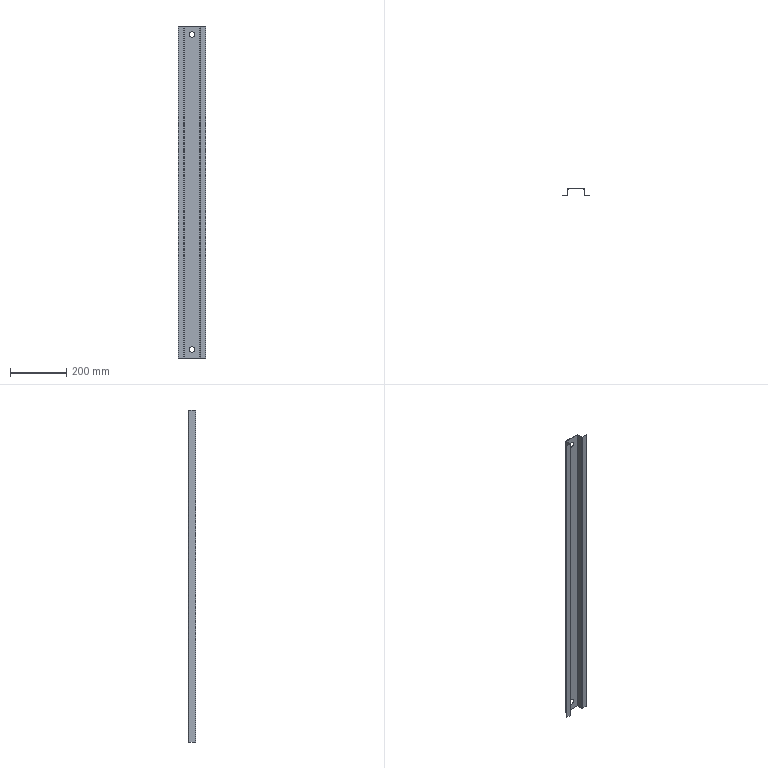Part | 1 solid | 42 faces | box 98.4 x 25 x 1180 mm | volume 135808 mm3 | plane 30 | cylinder 12 | commonest cylinder face diameters 2 x4 3.6 x4 20 x4
STEP:
#1=CARTESIAN_POINT('',(10.,-0.8,560.));
#2=VERTEX_POINT('',#1);
#3=CARTESIAN_POINT('',(-10.,-0.8,560.));
#4=VERTEX_POINT('',#3);
#5=CARTESIAN_POINT('',(0.,-0.8,560.));
#6=DIRECTION('',(0.,1.,0.));
#7=DIRECTION('',(-1.,0.,0.));
#8=AXIS2_PLACEMENT_3D('',#5,#6,#7);
#9=CIRCLE('',#8,10.);
#10=EDGE_CURVE('',#2,#4,#9,.T.);
#11=ORIENTED_EDGE('',*,*,#10,.F.);
#12=CARTESIAN_POINT('',(10.,0.,560.));
#13=VERTEX_POINT('',#12);
#14=CARTESIAN_POINT('',(10.,-10.,560.));
#15=DIRECTION('',(0.,1.,0.));
#16=VECTOR('',#15,1000.);
#17=LINE('',#14,#16);
#18=EDGE_CURVE('',#2,#13,#17,.T.);
#19=ORIENTED_EDGE('',*,*,#18,.T.);
#20=CARTESIAN_POINT('',(-10.,0.,560.));
#21=VERTEX_POINT('',#20);
#22=CARTESIAN_POINT('',(0.,0.,560.));
#23=DIRECTION('',(0.,1.,0.));
#24=DIRECTION('',(-1.,0.,0.));
#25=AXIS2_PLACEMENT_3D('',#22,#23,#24);
#26=CIRCLE('',#25,10.);
#27=EDGE_CURVE('',#13,#21,#26,.T.);
#28=ORIENTED_EDGE('',*,*,#27,.T.);
#29=CARTESIAN_POINT('',(-10.,-10.,560.));
#30=DIRECTION('',(0.,1.,0.));
#31=VECTOR('',#30,1000.);
#32=LINE('',#29,#31);
#33=EDGE_CURVE('',#4,#21,#32,.T.);
#34=ORIENTED_EDGE('',*,*,#33,.F.);
#35=EDGE_LOOP('',(#11,#19,#28,#34));
#36=FACE_OUTER_BOUND('',#35,.T.);
#37=CARTESIAN_POINT('',(0.,-10.,560.));
#38=DIRECTION('',(0.,1.,0.));
#39=DIRECTION('',(-1.,0.,0.));
#40=AXIS2_PLACEMENT_3D('',#37,#38,#39);
#41=CYLINDRICAL_SURFACE('',#40,10.);
#42=ADVANCED_FACE('',(#36),#41,.F.);
#43=CARTESIAN_POINT('',(10.,-0.8,-560.));
#44=VERTEX_POINT('',#43);
#45=CARTESIAN_POINT('',(-10.,-0.8,-560.));
#46=VERTEX_POINT('',#45);
#47=CARTESIAN_POINT('',(0.,-0.8,-560.));
#48=DIRECTION('',(0.,1.,0.));
#49=DIRECTION('',(-1.,0.,0.));
#50=AXIS2_PLACEMENT_3D('',#47,#48,#49);
#51=CIRCLE('',#50,10.);
#52=EDGE_CURVE('',#44,#46,#51,.T.);
#53=ORIENTED_EDGE('',*,*,#52,.F.);
#54=CARTESIAN_POINT('',(10.,0.,-560.));
#55=VERTEX_POINT('',#54);
#56=CARTESIAN_POINT('',(10.,-10.,-560.));
#57=DIRECTION('',(0.,1.,0.));
#58=VECTOR('',#57,1000.);
#59=LINE('',#56,#58);
#60=EDGE_CURVE('',#44,#55,#59,.T.);
#61=ORIENTED_EDGE('',*,*,#60,.T.);
#62=CARTESIAN_POINT('',(-10.,0.,-560.));
#63=VERTEX_POINT('',#62);
#64=CARTESIAN_POINT('',(0.,0.,-560.));
#65=DIRECTION('',(0.,1.,0.));
#66=DIRECTION('',(1.,0.,0.));
#67=AXIS2_PLACEMENT_3D('',#64,#65,#66);
#68=CIRCLE('',#67,10.);
#69=EDGE_CURVE('',#55,#63,#68,.T.);
#70=ORIENTED_EDGE('',*,*,#69,.T.);
#71=CARTESIAN_POINT('',(-10.,-10.,-560.));
#72=DIRECTION('',(0.,1.,0.));
#73=VECTOR('',#72,1000.);
#74=LINE('',#71,#73);
#75=EDGE_CURVE('',#46,#63,#74,.T.);
#76=ORIENTED_EDGE('',*,*,#75,.F.);
#77=EDGE_LOOP('',(#53,#61,#70,#76));
#78=FACE_OUTER_BOUND('',#77,.T.);
#79=CARTESIAN_POINT('',(0.,-10.,-560.));
#80=DIRECTION('',(0.,1.,0.));
#81=DIRECTION('',(-1.,0.,0.));
#82=AXIS2_PLACEMENT_3D('',#79,#80,#81);
#83=CYLINDRICAL_SURFACE('',#82,10.);
#84=ADVANCED_FACE('',(#78),#83,.F.);
#85=CARTESIAN_POINT('',(29.2,-23.2,-590.));
#86=VERTEX_POINT('',#85);
#87=CARTESIAN_POINT('',(29.2,-23.2,590.));
#88=VERTEX_POINT('',#87);
#89=CARTESIAN_POINT('',(29.2,-23.2,-590.));
#90=DIRECTION('',(0.,0.,1.));
#91=VECTOR('',#90,1000.);
#92=LINE('',#89,#91);
#93=EDGE_CURVE('',#86,#88,#92,.T.);
#94=ORIENTED_EDGE('',*,*,#93,.T.);
#95=CARTESIAN_POINT('',(29.2,-1.8,590.));
#96=VERTEX_POINT('',#95);
#97=CARTESIAN_POINT('',(29.2,0.,590.));
#98=DIRECTION('',(0.,-1.,0.));
#99=VECTOR('',#98,1000.);
#100=LINE('',#97,#99);
#101=EDGE_CURVE('',#96,#88,#100,.T.);
#102=ORIENTED_EDGE('',*,*,#101,.F.);
#103=CARTESIAN_POINT('',(29.2,-1.8,-590.));
#104=VERTEX_POINT('',#103);
#105=CARTESIAN_POINT('',(29.2,-1.8,590.));
#106=DIRECTION('',(0.,0.,-1.));
#107=VECTOR('',#106,1000.);
#108=LINE('',#105,#107);
#109=EDGE_CURVE('',#96,#104,#108,.T.);
#110=ORIENTED_EDGE('',*,*,#109,.T.);
#111=CARTESIAN_POINT('',(29.2,0.,-590.));
#112=DIRECTION('',(0.,-1.,0.));
#113=VECTOR('',#112,1000.);
#114=LINE('',#111,#113);
#115=EDGE_CURVE('',#104,#86,#114,.T.);
#116=ORIENTED_EDGE('',*,*,#115,.T.);
#117=EDGE_LOOP('',(#94,#102,#110,#116));
#118=FACE_OUTER_BOUND('',#117,.T.);
#119=CARTESIAN_POINT('',(29.2,0.,590.));
#120=DIRECTION('',(1.,0.,0.));
#121=DIRECTION('',(0.,1.,0.));
#122=AXIS2_PLACEMENT_3D('',#119,#120,#121);
#123=PLANE('',#122);
#124=ADVANCED_FACE('',(#118),#123,.F.);
#125=CARTESIAN_POINT('',(30.,-1.8,590.));
#126=VERTEX_POINT('',#125);
#127=CARTESIAN_POINT('',(30.,-23.2,590.));
#128=VERTEX_POINT('',#127);
#129=CARTESIAN_POINT('',(30.,0.,590.));
#130=DIRECTION('',(0.,-1.,0.));
#131=VECTOR('',#130,1000.);
#132=LINE('',#129,#131);
#133=EDGE_CURVE('',#126,#128,#132,.T.);
#134=ORIENTED_EDGE('',*,*,#133,.T.);
#135=CARTESIAN_POINT('',(30.,-23.2,-590.));
#136=VERTEX_POINT('',#135);
#137=CARTESIAN_POINT('',(30.,-23.2,-590.));
#138=DIRECTION('',(0.,0.,1.));
#139=VECTOR('',#138,1000.);
#140=LINE('',#137,#139);
#141=EDGE_CURVE('',#136,#128,#140,.T.);
#142=ORIENTED_EDGE('',*,*,#141,.F.);
#143=CARTESIAN_POINT('',(30.,-1.8,-590.));
#144=VERTEX_POINT('',#143);
#145=CARTESIAN_POINT('',(30.,0.,-590.));
#146=DIRECTION('',(0.,-1.,0.));
#147=VECTOR('',#146,1000.);
#148=LINE('',#145,#147);
#149=EDGE_CURVE('',#144,#136,#148,.T.);
#150=ORIENTED_EDGE('',*,*,#149,.F.);
#151=CARTESIAN_POINT('',(30.,-1.8,590.));
#152=DIRECTION('',(0.,0.,-1.));
#153=VECTOR('',#152,1000.);
#154=LINE('',#151,#153);
#155=EDGE_CURVE('',#126,#144,#154,.T.);
#156=ORIENTED_EDGE('',*,*,#155,.F.);
#157=EDGE_LOOP('',(#134,#142,#150,#156));
#158=FACE_OUTER_BOUND('',#157,.T.);
#159=CARTESIAN_POINT('',(30.,0.,590.));
#160=DIRECTION('',(1.,0.,0.));
#161=DIRECTION('',(0.,1.,0.));
#162=AXIS2_PLACEMENT_3D('',#159,#160,#161);
#163=PLANE('',#162);
#164=ADVANCED_FACE('',(#158),#163,.T.);
#165=CARTESIAN_POINT('',(30.,-23.2,-590.));
#166=DIRECTION('',(-1.,0.,0.));
#167=VECTOR('',#166,1000.);
#168=LINE('',#165,#167);
#169=EDGE_CURVE('',#136,#86,#168,.T.);
#170=ORIENTED_EDGE('',*,*,#169,.T.);
#171=ORIENTED_EDGE('',*,*,#115,.F.);
#172=CARTESIAN_POINT('',(29.2,-1.8,-590.));
#173=DIRECTION('',(1.,0.,0.));
#174=VECTOR('',#173,1000.);
#175=LINE('',#172,#174);
#176=EDGE_CURVE('',#104,#144,#175,.T.);
#177=ORIENTED_EDGE('',*,*,#176,.T.);
#178=ORIENTED_EDGE('',*,*,#149,.T.);
#179=EDGE_LOOP('',(#170,#171,#177,#178));
#180=FACE_OUTER_BOUND('',#179,.T.);
#181=CARTESIAN_POINT('',(28.2,-1.8,-590.));
#182=DIRECTION('',(0.,0.,1.));
#183=DIRECTION('',(1.,0.,0.));
#184=AXIS2_PLACEMENT_3D('',#181,#182,#183);
#185=PLANE('',#184);
#186=ADVANCED_FACE('',(#180),#185,.F.);
#187=CARTESIAN_POINT('',(-30.,-23.2,-590.));
#188=VERTEX_POINT('',#187);
#189=CARTESIAN_POINT('',(-30.,-1.8,-590.));
#190=VERTEX_POINT('',#189);
#191=CARTESIAN_POINT('',(-30.,-25.,-590.));
#192=DIRECTION('',(0.,1.,0.));
#193=VECTOR('',#192,1000.);
#194=LINE('',#191,#193);
#195=EDGE_CURVE('',#188,#190,#194,.T.);
#196=ORIENTED_EDGE('',*,*,#195,.F.);
#197=CARTESIAN_POINT('',(-30.,-23.2,590.));
#198=VERTEX_POINT('',#197);
#199=CARTESIAN_POINT('',(-30.,-23.2,590.));
#200=DIRECTION('',(0.,0.,-1.));
#201=VECTOR('',#200,1000.);
#202=LINE('',#199,#201);
#203=EDGE_CURVE('',#198,#188,#202,.T.);
#204=ORIENTED_EDGE('',*,*,#203,.F.);
#205=CARTESIAN_POINT('',(-30.,-1.8,590.));
#206=VERTEX_POINT('',#205);
#207=CARTESIAN_POINT('',(-30.,-25.,590.));
#208=DIRECTION('',(0.,1.,0.));
#209=VECTOR('',#208,1000.);
#210=LINE('',#207,#209);
#211=EDGE_CURVE('',#198,#206,#210,.T.);
#212=ORIENTED_EDGE('',*,*,#211,.T.);
#213=CARTESIAN_POINT('',(-30.,-1.8,590.));
#214=DIRECTION('',(0.,0.,-1.));
#215=VECTOR('',#214,1000.);
#216=LINE('',#213,#215);
#217=EDGE_CURVE('',#206,#190,#216,.T.);
#218=ORIENTED_EDGE('',*,*,#217,.T.);
#219=EDGE_LOOP('',(#196,#204,#212,#218));
#220=FACE_OUTER_BOUND('',#219,.T.);
#221=CARTESIAN_POINT('',(-30.,-25.,590.));
#222=DIRECTION('',(-1.,0.,0.));
#223=DIRECTION('',(0.,0.,1.));
#224=AXIS2_PLACEMENT_3D('',#221,#222,#223);
#225=PLANE('',#224);
#226=ADVANCED_FACE('',(#220),#225,.T.);
#227=CARTESIAN_POINT('',(-29.2,-23.2,590.));
#228=VERTEX_POINT('',#227);
#229=CARTESIAN_POINT('',(-29.2,-23.2,-590.));
#230=VERTEX_POINT('',#229);
#231=CARTESIAN_POINT('',(-29.2,-23.2,590.));
#232=DIRECTION('',(0.,0.,-1.));
#233=VECTOR('',#232,1000.);
#234=LINE('',#231,#233);
#235=EDGE_CURVE('',#228,#230,#234,.T.);
#236=ORIENTED_EDGE('',*,*,#235,.T.);
#237=CARTESIAN_POINT('',(-29.2,-1.8,-590.));
#238=VERTEX_POINT('',#237);
#239=CARTESIAN_POINT('',(-29.2,-25.,-590.));
#240=DIRECTION('',(0.,1.,0.));
#241=VECTOR('',#240,1000.);
#242=LINE('',#239,#241);
#243=EDGE_CURVE('',#230,#238,#242,.T.);
#244=ORIENTED_EDGE('',*,*,#243,.T.);
#245=CARTESIAN_POINT('',(-29.2,-1.8,590.));
#246=VERTEX_POINT('',#245);
#247=CARTESIAN_POINT('',(-29.2,-1.8,590.));
#248=DIRECTION('',(0.,0.,-1.));
#249=VECTOR('',#248,1000.);
#250=LINE('',#247,#249);
#251=EDGE_CURVE('',#246,#238,#250,.T.);
#252=ORIENTED_EDGE('',*,*,#251,.F.);
#253=CARTESIAN_POINT('',(-29.2,-25.,590.));
#254=DIRECTION('',(0.,1.,0.));
#255=VECTOR('',#254,1000.);
#256=LINE('',#253,#255);
#257=EDGE_CURVE('',#228,#246,#256,.T.);
#258=ORIENTED_EDGE('',*,*,#257,.F.);
#259=EDGE_LOOP('',(#236,#244,#252,#258));
#260=FACE_OUTER_BOUND('',#259,.T.);
#261=CARTESIAN_POINT('',(-29.2,-25.,590.));
#262=DIRECTION('',(-1.,0.,0.));
#263=DIRECTION('',(0.,0.,1.));
#264=AXIS2_PLACEMENT_3D('',#261,#262,#263);
#265=PLANE('',#264);
#266=ADVANCED_FACE('',(#260),#265,.F.);
#267=ORIENTED_EDGE('',*,*,#211,.F.);
#268=CARTESIAN_POINT('',(-30.,-23.2,590.));
#269=DIRECTION('',(1.,0.,0.));
#270=VECTOR('',#269,1000.);
#271=LINE('',#268,#270);
#272=EDGE_CURVE('',#198,#228,#271,.T.);
#273=ORIENTED_EDGE('',*,*,#272,.T.);
#274=ORIENTED_EDGE('',*,*,#257,.T.);
#275=CARTESIAN_POINT('',(-29.2,-1.8,590.));
#276=DIRECTION('',(-1.,0.,0.));
#277=VECTOR('',#276,1000.);
#278=LINE('',#275,#277);
#279=EDGE_CURVE('',#246,#206,#278,.T.);
#280=ORIENTED_EDGE('',*,*,#279,.T.);
#281=EDGE_LOOP('',(#267,#273,#274,#280));
#282=FACE_OUTER_BOUND('',#281,.T.);
#283=CARTESIAN_POINT('',(28.2,-1.8,590.));
#284=DIRECTION('',(0.,0.,1.));
#285=DIRECTION('',(1.,0.,0.));
#286=AXIS2_PLACEMENT_3D('',#283,#284,#285);
#287=PLANE('',#286);
#288=ADVANCED_FACE('',(#282),#287,.T.);
#289=CARTESIAN_POINT('',(-28.2,0.,590.));
#290=VERTEX_POINT('',#289);
#291=CARTESIAN_POINT('',(-28.2,-0.8,590.));
#292=VERTEX_POINT('',#291);
#293=CARTESIAN_POINT('',(-28.2,0.,590.));
#294=DIRECTION('',(0.,-1.,0.));
#295=VECTOR('',#294,1000.);
#296=LINE('',#293,#295);
#297=EDGE_CURVE('',#290,#292,#296,.T.);
#298=ORIENTED_EDGE('',*,*,#297,.F.);
#299=CARTESIAN_POINT('',(-28.2,-1.8,590.));
#300=DIRECTION('',(0.,0.,-1.));
#301=DIRECTION('',(1.,0.,0.));
#302=AXIS2_PLACEMENT_3D('',#299,#300,#301);
#303=CIRCLE('',#302,1.8);
#304=EDGE_CURVE('',#206,#290,#303,.T.);
#305=ORIENTED_EDGE('',*,*,#304,.F.);
#306=ORIENTED_EDGE('',*,*,#279,.F.);
#307=CARTESIAN_POINT('',(-28.2,-1.8,590.));
#308=DIRECTION('',(0.,0.,-1.));
#309=DIRECTION('',(1.,0.,0.));
#310=AXIS2_PLACEMENT_3D('',#307,#308,#309);
#311=CIRCLE('',#310,1.);
#312=EDGE_CURVE('',#246,#292,#311,.T.);
#313=ORIENTED_EDGE('',*,*,#312,.T.);
#314=EDGE_LOOP('',(#298,#305,#306,#313));
#315=FACE_OUTER_BOUND('',#314,.T.);
#316=CARTESIAN_POINT('',(-28.2,0.,590.));
#317=DIRECTION('',(0.,0.,1.));
#318=DIRECTION('',(1.,0.,0.));
#319=AXIS2_PLACEMENT_3D('',#316,#317,#318);
#320=PLANE('',#319);
#321=ADVANCED_FACE('',(#315),#320,.T.);
#322=CARTESIAN_POINT('',(28.2,0.,590.));
#323=VERTEX_POINT('',#322);
#324=CARTESIAN_POINT('',(-30.,0.,590.));
#325=DIRECTION('',(1.,0.,0.));
#326=VECTOR('',#325,1000.);
#327=LINE('',#324,#326);
#328=EDGE_CURVE('',#290,#323,#327,.T.);
#329=ORIENTED_EDGE('',*,*,#328,.F.);
#330=ORIENTED_EDGE('',*,*,#297,.T.);
#331=CARTESIAN_POINT('',(28.2,-0.8,590.));
#332=VERTEX_POINT('',#331);
#333=CARTESIAN_POINT('',(-30.,-0.8,590.));
#334=DIRECTION('',(1.,0.,0.));
#335=VECTOR('',#334,1000.);
#336=LINE('',#333,#335);
#337=EDGE_CURVE('',#292,#332,#336,.T.);
#338=ORIENTED_EDGE('',*,*,#337,.T.);
#339=CARTESIAN_POINT('',(28.2,-0.8,590.));
#340=DIRECTION('',(0.,1.,0.));
#341=VECTOR('',#340,1000.);
#342=LINE('',#339,#341);
#343=EDGE_CURVE('',#332,#323,#342,.T.);
#344=ORIENTED_EDGE('',*,*,#343,.T.);
#345=EDGE_LOOP('',(#329,#330,#338,#344));
#346=FACE_OUTER_BOUND('',#345,.T.);
#347=CARTESIAN_POINT('',(-29.2,-1.8,590.));
#348=DIRECTION('',(0.,0.,1.));
#349=DIRECTION('',(1.,0.,0.));
#350=AXIS2_PLACEMENT_3D('',#347,#348,#349);
#351=PLANE('',#350);
#352=ADVANCED_FACE('',(#346),#351,.T.);
#353=CARTESIAN_POINT('',(-30.,-1.8,-590.));
#354=DIRECTION('',(1.,0.,0.));
#355=VECTOR('',#354,1000.);
#356=LINE('',#353,#355);
#357=EDGE_CURVE('',#190,#238,#356,.T.);
#358=ORIENTED_EDGE('',*,*,#357,.F.);
#359=CARTESIAN_POINT('',(-28.2,0.,-590.));
#360=VERTEX_POINT('',#359);
#361=CARTESIAN_POINT('',(-28.2,-1.8,-590.));
#362=DIRECTION('',(0.,0.,-1.));
#363=DIRECTION('',(1.,0.,0.));
#364=AXIS2_PLACEMENT_3D('',#361,#362,#363);
#365=CIRCLE('',#364,1.8);
#366=EDGE_CURVE('',#190,#360,#365,.T.);
#367=ORIENTED_EDGE('',*,*,#366,.T.);
#368=CARTESIAN_POINT('',(-28.2,-0.8,-590.));
#369=VERTEX_POINT('',#368);
#370=CARTESIAN_POINT('',(-28.2,-0.8,-590.));
#371=DIRECTION('',(0.,1.,0.));
#372=VECTOR('',#371,1000.);
#373=LINE('',#370,#372);
#374=EDGE_CURVE('',#369,#360,#373,.T.);
#375=ORIENTED_EDGE('',*,*,#374,.F.);
#376=CARTESIAN_POINT('',(-28.2,-1.8,-590.));
#377=DIRECTION('',(0.,0.,-1.));
#378=DIRECTION('',(1.,0.,0.));
#379=AXIS2_PLACEMENT_3D('',#376,#377,#378);
#380=CIRCLE('',#379,1.);
#381=EDGE_CURVE('',#238,#369,#380,.T.);
#382=ORIENTED_EDGE('',*,*,#381,.F.);
#383=EDGE_LOOP('',(#358,#367,#375,#382));
#384=FACE_OUTER_BOUND('',#383,.T.);
#385=CARTESIAN_POINT('',(-30.,-1.8,-590.));
#386=DIRECTION('',(0.,0.,-1.));
#387=DIRECTION('',(-1.,0.,0.));
#388=AXIS2_PLACEMENT_3D('',#385,#386,#387);
#389=PLANE('',#388);
#390=ADVANCED_FACE('',(#384),#389,.T.);
#391=CARTESIAN_POINT('',(-30.,-23.2,-590.));
#392=DIRECTION('',(1.,0.,0.));
#393=VECTOR('',#392,1000.);
#394=LINE('',#391,#393);
#395=EDGE_CURVE('',#188,#230,#394,.T.);
#396=ORIENTED_EDGE('',*,*,#395,.F.);
#397=ORIENTED_EDGE('',*,*,#195,.T.);
#398=ORIENTED_EDGE('',*,*,#357,.T.);
#399=ORIENTED_EDGE('',*,*,#243,.F.);
#400=EDGE_LOOP('',(#396,#397,#398,#399));
#401=FACE_OUTER_BOUND('',#400,.T.);
#402=CARTESIAN_POINT('',(-28.2,-0.8,-590.));
#403=DIRECTION('',(0.,0.,-1.));
#404=DIRECTION('',(-1.,0.,0.));
#405=AXIS2_PLACEMENT_3D('',#402,#403,#404);
#406=PLANE('',#405);
#407=ADVANCED_FACE('',(#401),#406,.T.);
#408=CARTESIAN_POINT('',(30.,-1.8,590.));
#409=DIRECTION('',(-1.,0.,0.));
#410=VECTOR('',#409,1000.);
#411=LINE('',#408,#410);
#412=EDGE_CURVE('',#126,#96,#411,.T.);
#413=ORIENTED_EDGE('',*,*,#412,.F.);
#414=CARTESIAN_POINT('',(28.2,-1.8,590.));
#415=DIRECTION('',(0.,0.,-1.));
#416=DIRECTION('',(1.,0.,0.));
#417=AXIS2_PLACEMENT_3D('',#414,#415,#416);
#418=CIRCLE('',#417,1.8);
#419=EDGE_CURVE('',#323,#126,#418,.T.);
#420=ORIENTED_EDGE('',*,*,#419,.F.);
#421=ORIENTED_EDGE('',*,*,#343,.F.);
#422=CARTESIAN_POINT('',(28.2,-1.8,590.));
#423=DIRECTION('',(0.,0.,-1.));
#424=DIRECTION('',(1.,0.,0.));
#425=AXIS2_PLACEMENT_3D('',#422,#423,#424);
#426=CIRCLE('',#425,1.);
#427=EDGE_CURVE('',#332,#96,#426,.T.);
#428=ORIENTED_EDGE('',*,*,#427,.T.);
#429=EDGE_LOOP('',(#413,#420,#421,#428));
#430=FACE_OUTER_BOUND('',#429,.T.);
#431=CARTESIAN_POINT('',(30.,-1.8,590.));
#432=DIRECTION('',(0.,0.,1.));
#433=DIRECTION('',(1.,0.,0.));
#434=AXIS2_PLACEMENT_3D('',#431,#432,#433);
#435=PLANE('',#434);
#436=ADVANCED_FACE('',(#430),#435,.T.);
#437=CARTESIAN_POINT('',(30.,-23.2,590.));
#438=DIRECTION('',(-1.,0.,0.));
#439=VECTOR('',#438,1000.);
#440=LINE('',#437,#439);
#441=EDGE_CURVE('',#128,#88,#440,.T.);
#442=ORIENTED_EDGE('',*,*,#441,.F.);
#443=ORIENTED_EDGE('',*,*,#133,.F.);
#444=ORIENTED_EDGE('',*,*,#412,.T.);
#445=ORIENTED_EDGE('',*,*,#101,.T.);
#446=EDGE_LOOP('',(#442,#443,#444,#445));
#447=FACE_OUTER_BOUND('',#446,.T.);
#448=CARTESIAN_POINT('',(28.2,-0.8,590.));
#449=DIRECTION('',(0.,0.,1.));
#450=DIRECTION('',(1.,0.,0.));
#451=AXIS2_PLACEMENT_3D('',#448,#449,#450);
#452=PLANE('',#451);
#453=ADVANCED_FACE('',(#447),#452,.T.);
#454=CARTESIAN_POINT('',(28.2,0.,-590.));
#455=VERTEX_POINT('',#454);
#456=CARTESIAN_POINT('',(28.2,-0.8,-590.));
#457=VERTEX_POINT('',#456);
#458=CARTESIAN_POINT('',(28.2,0.,-590.));
#459=DIRECTION('',(0.,-1.,0.));
#460=VECTOR('',#459,1000.);
#461=LINE('',#458,#460);
#462=EDGE_CURVE('',#455,#457,#461,.T.);
#463=ORIENTED_EDGE('',*,*,#462,.F.);
#464=CARTESIAN_POINT('',(28.2,-1.8,-590.));
#465=DIRECTION('',(0.,0.,-1.));
#466=DIRECTION('',(1.,0.,0.));
#467=AXIS2_PLACEMENT_3D('',#464,#465,#466);
#468=CIRCLE('',#467,1.8);
#469=EDGE_CURVE('',#455,#144,#468,.T.);
#470=ORIENTED_EDGE('',*,*,#469,.T.);
#471=ORIENTED_EDGE('',*,*,#176,.F.);
#472=CARTESIAN_POINT('',(28.2,-1.8,-590.));
#473=DIRECTION('',(0.,0.,-1.));
#474=DIRECTION('',(1.,0.,0.));
#475=AXIS2_PLACEMENT_3D('',#472,#473,#474);
#476=CIRCLE('',#475,1.);
#477=EDGE_CURVE('',#457,#104,#476,.T.);
#478=ORIENTED_EDGE('',*,*,#477,.F.);
#479=EDGE_LOOP('',(#463,#470,#471,#478));
#480=FACE_OUTER_BOUND('',#479,.T.);
#481=CARTESIAN_POINT('',(28.2,0.,-590.));
#482=DIRECTION('',(0.,0.,-1.));
#483=DIRECTION('',(-1.,0.,0.));
#484=AXIS2_PLACEMENT_3D('',#481,#482,#483);
#485=PLANE('',#484);
#486=ADVANCED_FACE('',(#480),#485,.T.);
#487=CARTESIAN_POINT('',(-30.,0.,-590.));
#488=DIRECTION('',(1.,0.,0.));
#489=VECTOR('',#488,1000.);
#490=LINE('',#487,#489);
#491=EDGE_CURVE('',#360,#455,#490,.T.);
#492=ORIENTED_EDGE('',*,*,#491,.T.);
#493=ORIENTED_EDGE('',*,*,#462,.T.);
#494=CARTESIAN_POINT('',(-30.,-0.8,-590.));
#495=DIRECTION('',(1.,0.,0.));
#496=VECTOR('',#495,1000.);
#497=LINE('',#494,#496);
#498=EDGE_CURVE('',#369,#457,#497,.T.);
#499=ORIENTED_EDGE('',*,*,#498,.F.);
#500=ORIENTED_EDGE('',*,*,#374,.T.);
#501=EDGE_LOOP('',(#492,#493,#499,#500));
#502=FACE_OUTER_BOUND('',#501,.T.);
#503=CARTESIAN_POINT('',(29.2,-1.8,-590.));
#504=DIRECTION('',(0.,0.,-1.));
#505=DIRECTION('',(-1.,0.,0.));
#506=AXIS2_PLACEMENT_3D('',#503,#504,#505);
#507=PLANE('',#506);
#508=ADVANCED_FACE('',(#502),#507,.T.);
#509=ORIENTED_EDGE('',*,*,#469,.F.);
#510=CARTESIAN_POINT('',(28.2,0.,590.));
#511=DIRECTION('',(0.,0.,-1.));
#512=VECTOR('',#511,1000.);
#513=LINE('',#510,#512);
#514=EDGE_CURVE('',#323,#455,#513,.T.);
#515=ORIENTED_EDGE('',*,*,#514,.F.);
#516=ORIENTED_EDGE('',*,*,#419,.T.);
#517=ORIENTED_EDGE('',*,*,#155,.T.);
#518=EDGE_LOOP('',(#509,#515,#516,#517));
#519=FACE_OUTER_BOUND('',#518,.T.);
#520=CARTESIAN_POINT('',(28.2,-1.8,590.));
#521=DIRECTION('',(0.,0.,-1.));
#522=DIRECTION('',(-1.,0.,0.));
#523=AXIS2_PLACEMENT_3D('',#520,#521,#522);
#524=CYLINDRICAL_SURFACE('',#523,1.8);
#525=ADVANCED_FACE('',(#519),#524,.T.);
#526=CARTESIAN_POINT('',(0.,0.,560.));
#527=DIRECTION('',(0.,1.,0.));
#528=DIRECTION('',(-1.,0.,0.));
#529=AXIS2_PLACEMENT_3D('',#526,#527,#528);
#530=CIRCLE('',#529,10.);
#531=EDGE_CURVE('',#21,#13,#530,.T.);
#532=ORIENTED_EDGE('',*,*,#531,.F.);
#533=ORIENTED_EDGE('',*,*,#27,.F.);
#534=EDGE_LOOP('',(#532,#533));
#535=FACE_BOUND('',#534,.T.);
#536=CARTESIAN_POINT('',(0.,0.,-560.));
#537=DIRECTION('',(0.,1.,0.));
#538=DIRECTION('',(1.,0.,0.));
#539=AXIS2_PLACEMENT_3D('',#536,#537,#538);
#540=CIRCLE('',#539,10.);
#541=EDGE_CURVE('',#63,#55,#540,.T.);
#542=ORIENTED_EDGE('',*,*,#541,.F.);
#543=ORIENTED_EDGE('',*,*,#69,.F.);
#544=EDGE_LOOP('',(#542,#543));
#545=FACE_BOUND('',#544,.T.);
#546=ORIENTED_EDGE('',*,*,#491,.F.);
#547=CARTESIAN_POINT('',(-28.2,0.,590.));
#548=DIRECTION('',(0.,0.,-1.));
#549=VECTOR('',#548,1000.);
#550=LINE('',#547,#549);
#551=EDGE_CURVE('',#290,#360,#550,.T.);
#552=ORIENTED_EDGE('',*,*,#551,.F.);
#553=ORIENTED_EDGE('',*,*,#328,.T.);
#554=ORIENTED_EDGE('',*,*,#514,.T.);
#555=EDGE_LOOP('',(#546,#552,#553,#554));
#556=FACE_OUTER_BOUND('',#555,.T.);
#557=CARTESIAN_POINT('',(-30.,0.,590.));
#558=DIRECTION('',(0.,1.,0.));
#559=DIRECTION('',(-1.,0.,0.));
#560=AXIS2_PLACEMENT_3D('',#557,#558,#559);
#561=PLANE('',#560);
#562=ADVANCED_FACE('',(#535,#545,#556),#561,.T.);
#563=ORIENTED_EDGE('',*,*,#366,.F.);
#564=ORIENTED_EDGE('',*,*,#217,.F.);
#565=ORIENTED_EDGE('',*,*,#304,.T.);
#566=ORIENTED_EDGE('',*,*,#551,.T.);
#567=EDGE_LOOP('',(#563,#564,#565,#566));
#568=FACE_OUTER_BOUND('',#567,.T.);
#569=CARTESIAN_POINT('',(-28.2,-1.8,590.));
#570=DIRECTION('',(0.,0.,-1.));
#571=DIRECTION('',(-1.,0.,0.));
#572=AXIS2_PLACEMENT_3D('',#569,#570,#571);
#573=CYLINDRICAL_SURFACE('',#572,1.8);
#574=ADVANCED_FACE('',(#568),#573,.T.);
#575=ORIENTED_EDGE('',*,*,#381,.T.);
#576=CARTESIAN_POINT('',(-28.2,-0.8,590.));
#577=DIRECTION('',(0.,0.,-1.));
#578=VECTOR('',#577,1000.);
#579=LINE('',#576,#578);
#580=EDGE_CURVE('',#292,#369,#579,.T.);
#581=ORIENTED_EDGE('',*,*,#580,.F.);
#582=ORIENTED_EDGE('',*,*,#312,.F.);
#583=ORIENTED_EDGE('',*,*,#251,.T.);
#584=EDGE_LOOP('',(#575,#581,#582,#583));
#585=FACE_OUTER_BOUND('',#584,.T.);
#586=CARTESIAN_POINT('',(-28.2,-1.8,590.));
#587=DIRECTION('',(0.,0.,-1.));
#588=DIRECTION('',(-1.,0.,0.));
#589=AXIS2_PLACEMENT_3D('',#586,#587,#588);
#590=CYLINDRICAL_SURFACE('',#589,1.);
#591=ADVANCED_FACE('',(#585),#590,.F.);
#592=CARTESIAN_POINT('',(0.,-0.8,560.));
#593=DIRECTION('',(0.,1.,0.));
#594=DIRECTION('',(-1.,0.,0.));
#595=AXIS2_PLACEMENT_3D('',#592,#593,#594);
#596=CIRCLE('',#595,10.);
#597=EDGE_CURVE('',#4,#2,#596,.T.);
#598=ORIENTED_EDGE('',*,*,#597,.T.);
#599=ORIENTED_EDGE('',*,*,#10,.T.);
#600=EDGE_LOOP('',(#598,#599));
#601=FACE_BOUND('',#600,.T.);
#602=CARTESIAN_POINT('',(0.,-0.8,-560.));
#603=DIRECTION('',(0.,1.,0.));
#604=DIRECTION('',(-1.,0.,0.));
#605=AXIS2_PLACEMENT_3D('',#602,#603,#604);
#606=CIRCLE('',#605,10.);
#607=EDGE_CURVE('',#46,#44,#606,.T.);
#608=ORIENTED_EDGE('',*,*,#607,.T.);
#609=ORIENTED_EDGE('',*,*,#52,.T.);
#610=EDGE_LOOP('',(#608,#609));
#611=FACE_BOUND('',#610,.T.);
#612=ORIENTED_EDGE('',*,*,#498,.T.);
#613=CARTESIAN_POINT('',(28.2,-0.8,590.));
#614=DIRECTION('',(0.,0.,-1.));
#615=VECTOR('',#614,1000.);
#616=LINE('',#613,#615);
#617=EDGE_CURVE('',#332,#457,#616,.T.);
#618=ORIENTED_EDGE('',*,*,#617,.F.);
#619=ORIENTED_EDGE('',*,*,#337,.F.);
#620=ORIENTED_EDGE('',*,*,#580,.T.);
#621=EDGE_LOOP('',(#612,#618,#619,#620));
#622=FACE_OUTER_BOUND('',#621,.T.);
#623=CARTESIAN_POINT('',(-30.,-0.8,590.));
#624=DIRECTION('',(0.,1.,0.));
#625=DIRECTION('',(-1.,0.,0.));
#626=AXIS2_PLACEMENT_3D('',#623,#624,#625);
#627=PLANE('',#626);
#628=ADVANCED_FACE('',(#601,#611,#622),#627,.F.);
#629=ORIENTED_EDGE('',*,*,#477,.T.);
#630=ORIENTED_EDGE('',*,*,#109,.F.);
#631=ORIENTED_EDGE('',*,*,#427,.F.);
#632=ORIENTED_EDGE('',*,*,#617,.T.);
#633=EDGE_LOOP('',(#629,#630,#631,#632));
#634=FACE_OUTER_BOUND('',#633,.T.);
#635=CARTESIAN_POINT('',(28.2,-1.8,590.));
#636=DIRECTION('',(0.,0.,-1.));
#637=DIRECTION('',(-1.,0.,0.));
#638=AXIS2_PLACEMENT_3D('',#635,#636,#637);
#639=CYLINDRICAL_SURFACE('',#638,1.);
#640=ADVANCED_FACE('',(#634),#639,.F.);
#641=CARTESIAN_POINT('',(-31.,-24.2,-590.));
#642=VERTEX_POINT('',#641);
#643=CARTESIAN_POINT('',(-31.,-25.,-590.));
#644=VERTEX_POINT('',#643);
#645=CARTESIAN_POINT('',(-31.,-25.,-590.));
#646=DIRECTION('',(0.,-1.,0.));
#647=VECTOR('',#646,1000.);
#648=LINE('',#645,#647);
#649=EDGE_CURVE('',#642,#644,#648,.T.);
#650=ORIENTED_EDGE('',*,*,#649,.F.);
#651=CARTESIAN_POINT('',(-31.,-23.2,-590.));
#652=DIRECTION('',(0.,0.,-1.));
#653=DIRECTION('',(1.,0.,0.));
#654=AXIS2_PLACEMENT_3D('',#651,#652,#653);
#655=CIRCLE('',#654,1.);
#656=EDGE_CURVE('',#188,#642,#655,.T.);
#657=ORIENTED_EDGE('',*,*,#656,.F.);
#658=ORIENTED_EDGE('',*,*,#395,.T.);
#659=CARTESIAN_POINT('',(-31.,-23.2,-590.));
#660=DIRECTION('',(0.,0.,-1.));
#661=DIRECTION('',(1.,0.,0.));
#662=AXIS2_PLACEMENT_3D('',#659,#660,#661);
#663=CIRCLE('',#662,1.8);
#664=EDGE_CURVE('',#230,#644,#663,.T.);
#665=ORIENTED_EDGE('',*,*,#664,.T.);
#666=EDGE_LOOP('',(#650,#657,#658,#665));
#667=FACE_OUTER_BOUND('',#666,.T.);
#668=CARTESIAN_POINT('',(-31.,-23.2,-590.));
#669=DIRECTION('',(0.,0.,-1.));
#670=DIRECTION('',(-1.,0.,0.));
#671=AXIS2_PLACEMENT_3D('',#668,#669,#670);
#672=PLANE('',#671);
#673=ADVANCED_FACE('',(#667),#672,.T.);
#674=CARTESIAN_POINT('',(-31.,-24.2,590.));
#675=VERTEX_POINT('',#674);
#676=CARTESIAN_POINT('',(-31.,-23.2,590.));
#677=DIRECTION('',(0.,0.,1.));
#678=DIRECTION('',(1.,0.,0.));
#679=AXIS2_PLACEMENT_3D('',#676,#677,#678);
#680=CIRCLE('',#679,1.);
#681=EDGE_CURVE('',#675,#198,#680,.T.);
#682=ORIENTED_EDGE('',*,*,#681,.F.);
#683=CARTESIAN_POINT('',(-31.,-25.,590.));
#684=VERTEX_POINT('',#683);
#685=CARTESIAN_POINT('',(-31.,-24.2,590.));
#686=DIRECTION('',(0.,-1.,0.));
#687=VECTOR('',#686,1000.);
#688=LINE('',#685,#687);
#689=EDGE_CURVE('',#675,#684,#688,.T.);
#690=ORIENTED_EDGE('',*,*,#689,.T.);
#691=CARTESIAN_POINT('',(-31.,-23.2,590.));
#692=DIRECTION('',(0.,0.,1.));
#693=DIRECTION('',(1.,0.,0.));
#694=AXIS2_PLACEMENT_3D('',#691,#692,#693);
#695=CIRCLE('',#694,1.8);
#696=EDGE_CURVE('',#684,#228,#695,.T.);
#697=ORIENTED_EDGE('',*,*,#696,.T.);
#698=ORIENTED_EDGE('',*,*,#272,.F.);
#699=EDGE_LOOP('',(#682,#690,#697,#698));
#700=FACE_OUTER_BOUND('',#699,.T.);
#701=CARTESIAN_POINT('',(-31.,-23.2,590.));
#702=DIRECTION('',(0.,0.,-1.));
#703=DIRECTION('',(-1.,0.,0.));
#704=AXIS2_PLACEMENT_3D('',#701,#702,#703);
#705=PLANE('',#704);
#706=ADVANCED_FACE('',(#700),#705,.F.);
#707=ORIENTED_EDGE('',*,*,#235,.F.);
#708=ORIENTED_EDGE('',*,*,#696,.F.);
#709=CARTESIAN_POINT('',(-31.,-25.,-590.));
#710=DIRECTION('',(0.,0.,-1.));
#711=VECTOR('',#710,1000.);
#712=LINE('',#709,#711);
#713=EDGE_CURVE('',#684,#644,#712,.T.);
#714=ORIENTED_EDGE('',*,*,#713,.T.);
#715=ORIENTED_EDGE('',*,*,#664,.F.);
#716=EDGE_LOOP('',(#707,#708,#714,#715));
#717=FACE_OUTER_BOUND('',#716,.T.);
#718=CARTESIAN_POINT('',(-31.,-23.2,590.));
#719=DIRECTION('',(0.,0.,1.));
#720=DIRECTION('',(0.,-1.,0.));
#721=AXIS2_PLACEMENT_3D('',#718,#719,#720);
#722=CYLINDRICAL_SURFACE('',#721,1.8);
#723=ADVANCED_FACE('',(#717),#722,.T.);
#724=ORIENTED_EDGE('',*,*,#203,.T.);
#725=ORIENTED_EDGE('',*,*,#656,.T.);
#726=CARTESIAN_POINT('',(-31.,-24.2,-590.));
#727=DIRECTION('',(0.,0.,1.));
#728=VECTOR('',#727,1000.);
#729=LINE('',#726,#728);
#730=EDGE_CURVE('',#642,#675,#729,.T.);
#731=ORIENTED_EDGE('',*,*,#730,.T.);
#732=ORIENTED_EDGE('',*,*,#681,.T.);
#733=EDGE_LOOP('',(#724,#725,#731,#732));
#734=FACE_OUTER_BOUND('',#733,.T.);
#735=CARTESIAN_POINT('',(-31.,-23.2,590.));
#736=DIRECTION('',(0.,0.,1.));
#737=DIRECTION('',(0.,-1.,0.));
#738=AXIS2_PLACEMENT_3D('',#735,#736,#737);
#739=CYLINDRICAL_SURFACE('',#738,1.);
#740=ADVANCED_FACE('',(#734),#739,.F.);
#741=ORIENTED_EDGE('',*,*,#689,.F.);
#742=CARTESIAN_POINT('',(-49.2,-24.2,590.));
#743=VERTEX_POINT('',#742);
#744=CARTESIAN_POINT('',(-49.2,-24.2,590.));
#745=DIRECTION('',(-1.,0.,0.));
#746=VECTOR('',#745,1000.);
#747=LINE('',#744,#746);
#748=EDGE_CURVE('',#675,#743,#747,.T.);
#749=ORIENTED_EDGE('',*,*,#748,.T.);
#750=CARTESIAN_POINT('',(-49.2,-25.,590.));
#751=VERTEX_POINT('',#750);
#752=CARTESIAN_POINT('',(-49.2,-25.,590.));
#753=DIRECTION('',(0.,1.,0.));
#754=VECTOR('',#753,1000.);
#755=LINE('',#752,#754);
#756=EDGE_CURVE('',#751,#743,#755,.T.);
#757=ORIENTED_EDGE('',*,*,#756,.F.);
#758=CARTESIAN_POINT('',(0.,-25.,590.));
#759=DIRECTION('',(-1.,0.,0.));
#760=VECTOR('',#759,1000.);
#761=LINE('',#758,#760);
#762=EDGE_CURVE('',#684,#751,#761,.T.);
#763=ORIENTED_EDGE('',*,*,#762,.F.);
#764=EDGE_LOOP('',(#741,#749,#757,#763));
#765=FACE_OUTER_BOUND('',#764,.T.);
#766=CARTESIAN_POINT('',(-49.2,-25.,590.));
#767=DIRECTION('',(0.,0.,-1.));
#768=DIRECTION('',(-1.,0.,0.));
#769=AXIS2_PLACEMENT_3D('',#766,#767,#768);
#770=PLANE('',#769);
#771=ADVANCED_FACE('',(#765),#770,.F.);
#772=ORIENTED_EDGE('',*,*,#649,.T.);
#773=CARTESIAN_POINT('',(-49.2,-25.,-590.));
#774=VERTEX_POINT('',#773);
#775=CARTESIAN_POINT('',(0.,-25.,-590.));
#776=DIRECTION('',(1.,0.,0.));
#777=VECTOR('',#776,1000.);
#778=LINE('',#775,#777);
#779=EDGE_CURVE('',#774,#644,#778,.T.);
#780=ORIENTED_EDGE('',*,*,#779,.F.);
#781=CARTESIAN_POINT('',(-49.2,-24.2,-590.));
#782=VERTEX_POINT('',#781);
#783=CARTESIAN_POINT('',(-49.2,-25.,-590.));
#784=DIRECTION('',(0.,1.,0.));
#785=VECTOR('',#784,1000.);
#786=LINE('',#783,#785);
#787=EDGE_CURVE('',#774,#782,#786,.T.);
#788=ORIENTED_EDGE('',*,*,#787,.T.);
#789=CARTESIAN_POINT('',(-30.,-24.2,-590.));
#790=DIRECTION('',(1.,0.,0.));
#791=VECTOR('',#790,1000.);
#792=LINE('',#789,#791);
#793=EDGE_CURVE('',#782,#642,#792,.T.);
#794=ORIENTED_EDGE('',*,*,#793,.T.);
#795=EDGE_LOOP('',(#772,#780,#788,#794));
#796=FACE_OUTER_BOUND('',#795,.T.);
#797=CARTESIAN_POINT('',(-30.,-25.,-590.));
#798=DIRECTION('',(0.,0.,1.));
#799=DIRECTION('',(1.,0.,0.));
#800=AXIS2_PLACEMENT_3D('',#797,#798,#799);
#801=PLANE('',#800);
#802=ADVANCED_FACE('',(#796),#801,.F.);
#803=ORIENTED_EDGE('',*,*,#713,.F.);
#804=ORIENTED_EDGE('',*,*,#762,.T.);
#805=CARTESIAN_POINT('',(-49.2,-25.,0.));
#806=DIRECTION('',(0.,0.,-1.));
#807=VECTOR('',#806,1000.);
#808=LINE('',#805,#807);
#809=EDGE_CURVE('',#751,#774,#808,.T.);
#810=ORIENTED_EDGE('',*,*,#809,.T.);
#811=ORIENTED_EDGE('',*,*,#779,.T.);
#812=EDGE_LOOP('',(#803,#804,#810,#811));
#813=FACE_OUTER_BOUND('',#812,.T.);
#814=CARTESIAN_POINT('',(0.,-25.,0.));
#815=DIRECTION('',(0.,1.,0.));
#816=DIRECTION('',(-1.,0.,0.));
#817=AXIS2_PLACEMENT_3D('',#814,#815,#816);
#818=PLANE('',#817);
#819=ADVANCED_FACE('',(#813),#818,.F.);
#820=ORIENTED_EDGE('',*,*,#748,.F.);
#821=ORIENTED_EDGE('',*,*,#730,.F.);
#822=ORIENTED_EDGE('',*,*,#793,.F.);
#823=CARTESIAN_POINT('',(-49.2,-24.2,-590.));
#824=DIRECTION('',(0.,0.,-1.));
#825=VECTOR('',#824,1000.);
#826=LINE('',#823,#825);
#827=EDGE_CURVE('',#743,#782,#826,.T.);
#828=ORIENTED_EDGE('',*,*,#827,.F.);
#829=EDGE_LOOP('',(#820,#821,#822,#828));
#830=FACE_OUTER_BOUND('',#829,.T.);
#831=CARTESIAN_POINT('',(0.,-24.2,0.));
#832=DIRECTION('',(0.,1.,0.));
#833=DIRECTION('',(-1.,0.,0.));
#834=AXIS2_PLACEMENT_3D('',#831,#832,#833);
#835=PLANE('',#834);
#836=ADVANCED_FACE('',(#830),#835,.T.);
#837=ORIENTED_EDGE('',*,*,#827,.T.);
#838=ORIENTED_EDGE('',*,*,#787,.F.);
#839=ORIENTED_EDGE('',*,*,#809,.F.);
#840=ORIENTED_EDGE('',*,*,#756,.T.);
#841=EDGE_LOOP('',(#837,#838,#839,#840));
#842=FACE_OUTER_BOUND('',#841,.T.);
#843=CARTESIAN_POINT('',(-49.2,-25.,-590.));
#844=DIRECTION('',(1.,0.,0.));
#845=DIRECTION('',(0.,1.,0.));
#846=AXIS2_PLACEMENT_3D('',#843,#844,#845);
#847=PLANE('',#846);
#848=ADVANCED_FACE('',(#842),#847,.F.);
#849=CARTESIAN_POINT('',(31.,-24.2,590.));
#850=VERTEX_POINT('',#849);
#851=CARTESIAN_POINT('',(31.,-25.,590.));
#852=VERTEX_POINT('',#851);
#853=CARTESIAN_POINT('',(31.,-25.,590.));
#854=DIRECTION('',(0.,-1.,0.));
#855=VECTOR('',#854,1000.);
#856=LINE('',#853,#855);
#857=EDGE_CURVE('',#850,#852,#856,.T.);
#858=ORIENTED_EDGE('',*,*,#857,.F.);
#859=CARTESIAN_POINT('',(31.,-23.2,590.));
#860=DIRECTION('',(0.,0.,1.));
#861=DIRECTION('',(-1.,0.,0.));
#862=AXIS2_PLACEMENT_3D('',#859,#860,#861);
#863=CIRCLE('',#862,1.);
#864=EDGE_CURVE('',#128,#850,#863,.T.);
#865=ORIENTED_EDGE('',*,*,#864,.F.);
#866=ORIENTED_EDGE('',*,*,#441,.T.);
#867=CARTESIAN_POINT('',(31.,-23.2,590.));
#868=DIRECTION('',(0.,0.,1.));
#869=DIRECTION('',(-1.,0.,0.));
#870=AXIS2_PLACEMENT_3D('',#867,#868,#869);
#871=CIRCLE('',#870,1.8);
#872=EDGE_CURVE('',#88,#852,#871,.T.);
#873=ORIENTED_EDGE('',*,*,#872,.T.);
#874=EDGE_LOOP('',(#858,#865,#866,#873));
#875=FACE_OUTER_BOUND('',#874,.T.);
#876=CARTESIAN_POINT('',(31.,-23.2,590.));
#877=DIRECTION('',(0.,0.,1.));
#878=DIRECTION('',(1.,0.,0.));
#879=AXIS2_PLACEMENT_3D('',#876,#877,#878);
#880=PLANE('',#879);
#881=ADVANCED_FACE('',(#875),#880,.T.);
#882=CARTESIAN_POINT('',(31.,-24.2,-590.));
#883=VERTEX_POINT('',#882);
#884=CARTESIAN_POINT('',(31.,-23.2,-590.));
#885=DIRECTION('',(0.,0.,-1.));
#886=DIRECTION('',(-1.,0.,0.));
#887=AXIS2_PLACEMENT_3D('',#884,#885,#886);
#888=CIRCLE('',#887,1.);
#889=EDGE_CURVE('',#883,#136,#888,.T.);
#890=ORIENTED_EDGE('',*,*,#889,.F.);
#891=CARTESIAN_POINT('',(31.,-25.,-590.));
#892=VERTEX_POINT('',#891);
#893=CARTESIAN_POINT('',(31.,-24.2,-590.));
#894=DIRECTION('',(0.,-1.,0.));
#895=VECTOR('',#894,1000.);
#896=LINE('',#893,#895);
#897=EDGE_CURVE('',#883,#892,#896,.T.);
#898=ORIENTED_EDGE('',*,*,#897,.T.);
#899=CARTESIAN_POINT('',(31.,-23.2,-590.));
#900=DIRECTION('',(0.,0.,-1.));
#901=DIRECTION('',(-1.,0.,0.));
#902=AXIS2_PLACEMENT_3D('',#899,#900,#901);
#903=CIRCLE('',#902,1.8);
#904=EDGE_CURVE('',#892,#86,#903,.T.);
#905=ORIENTED_EDGE('',*,*,#904,.T.);
#906=ORIENTED_EDGE('',*,*,#169,.F.);
#907=EDGE_LOOP('',(#890,#898,#905,#906));
#908=FACE_OUTER_BOUND('',#907,.T.);
#909=CARTESIAN_POINT('',(31.,-23.2,-590.));
#910=DIRECTION('',(0.,0.,1.));
#911=DIRECTION('',(1.,0.,0.));
#912=AXIS2_PLACEMENT_3D('',#909,#910,#911);
#913=PLANE('',#912);
#914=ADVANCED_FACE('',(#908),#913,.F.);
#915=ORIENTED_EDGE('',*,*,#93,.F.);
#916=ORIENTED_EDGE('',*,*,#904,.F.);
#917=CARTESIAN_POINT('',(31.,-25.,590.));
#918=DIRECTION('',(0.,0.,1.));
#919=VECTOR('',#918,1000.);
#920=LINE('',#917,#919);
#921=EDGE_CURVE('',#892,#852,#920,.T.);
#922=ORIENTED_EDGE('',*,*,#921,.T.);
#923=ORIENTED_EDGE('',*,*,#872,.F.);
#924=EDGE_LOOP('',(#915,#916,#922,#923));
#925=FACE_OUTER_BOUND('',#924,.T.);
#926=CARTESIAN_POINT('',(31.,-23.2,-590.));
#927=DIRECTION('',(0.,0.,-1.));
#928=DIRECTION('',(0.,-1.,0.));
#929=AXIS2_PLACEMENT_3D('',#926,#927,#928);
#930=CYLINDRICAL_SURFACE('',#929,1.8);
#931=ADVANCED_FACE('',(#925),#930,.T.);
#932=ORIENTED_EDGE('',*,*,#141,.T.);
#933=ORIENTED_EDGE('',*,*,#864,.T.);
#934=CARTESIAN_POINT('',(31.,-24.2,590.));
#935=DIRECTION('',(0.,0.,-1.));
#936=VECTOR('',#935,1000.);
#937=LINE('',#934,#936);
#938=EDGE_CURVE('',#850,#883,#937,.T.);
#939=ORIENTED_EDGE('',*,*,#938,.T.);
#940=ORIENTED_EDGE('',*,*,#889,.T.);
#941=EDGE_LOOP('',(#932,#933,#939,#940));
#942=FACE_OUTER_BOUND('',#941,.T.);
#943=CARTESIAN_POINT('',(31.,-23.2,-590.));
#944=DIRECTION('',(0.,0.,-1.));
#945=DIRECTION('',(0.,-1.,0.));
#946=AXIS2_PLACEMENT_3D('',#943,#944,#945);
#947=CYLINDRICAL_SURFACE('',#946,1.);
#948=ADVANCED_FACE('',(#942),#947,.F.);
#949=ORIENTED_EDGE('',*,*,#857,.T.);
#950=CARTESIAN_POINT('',(49.2,-25.,590.));
#951=VERTEX_POINT('',#950);
#952=CARTESIAN_POINT('',(0.,-25.,590.));
#953=DIRECTION('',(-1.,0.,0.));
#954=VECTOR('',#953,1000.);
#955=LINE('',#952,#954);
#956=EDGE_CURVE('',#951,#852,#955,.T.);
#957=ORIENTED_EDGE('',*,*,#956,.F.);
#958=CARTESIAN_POINT('',(49.2,-24.2,590.));
#959=VERTEX_POINT('',#958);
#960=CARTESIAN_POINT('',(49.2,-25.,590.));
#961=DIRECTION('',(0.,1.,0.));
#962=VECTOR('',#961,1000.);
#963=LINE('',#960,#962);
#964=EDGE_CURVE('',#951,#959,#963,.T.);
#965=ORIENTED_EDGE('',*,*,#964,.T.);
#966=CARTESIAN_POINT('',(30.,-24.2,590.));
#967=DIRECTION('',(-1.,0.,0.));
#968=VECTOR('',#967,1000.);
#969=LINE('',#966,#968);
#970=EDGE_CURVE('',#959,#850,#969,.T.);
#971=ORIENTED_EDGE('',*,*,#970,.T.);
#972=EDGE_LOOP('',(#949,#957,#965,#971));
#973=FACE_OUTER_BOUND('',#972,.T.);
#974=CARTESIAN_POINT('',(30.,-25.,590.));
#975=DIRECTION('',(0.,0.,-1.));
#976=DIRECTION('',(-1.,0.,0.));
#977=AXIS2_PLACEMENT_3D('',#974,#975,#976);
#978=PLANE('',#977);
#979=ADVANCED_FACE('',(#973),#978,.F.);
#980=ORIENTED_EDGE('',*,*,#897,.F.);
#981=CARTESIAN_POINT('',(49.2,-24.2,-590.));
#982=VERTEX_POINT('',#981);
#983=CARTESIAN_POINT('',(49.2,-24.2,-590.));
#984=DIRECTION('',(1.,0.,0.));
#985=VECTOR('',#984,1000.);
#986=LINE('',#983,#985);
#987=EDGE_CURVE('',#883,#982,#986,.T.);
#988=ORIENTED_EDGE('',*,*,#987,.T.);
#989=CARTESIAN_POINT('',(49.2,-25.,-590.));
#990=VERTEX_POINT('',#989);
#991=CARTESIAN_POINT('',(49.2,-25.,-590.));
#992=DIRECTION('',(0.,1.,0.));
#993=VECTOR('',#992,1000.);
#994=LINE('',#991,#993);
#995=EDGE_CURVE('',#990,#982,#994,.T.);
#996=ORIENTED_EDGE('',*,*,#995,.F.);
#997=CARTESIAN_POINT('',(0.,-25.,-590.));
#998=DIRECTION('',(1.,0.,0.));
#999=VECTOR('',#998,1000.);
#1000=LINE('',#997,#999);
#1001=EDGE_CURVE('',#892,#990,#1000,.T.);
#1002=ORIENTED_EDGE('',*,*,#1001,.F.);
#1003=EDGE_LOOP('',(#980,#988,#996,#1002));
#1004=FACE_OUTER_BOUND('',#1003,.T.);
#1005=CARTESIAN_POINT('',(49.2,-25.,-590.));
#1006=DIRECTION('',(0.,0.,1.));
#1007=DIRECTION('',(1.,0.,0.));
#1008=AXIS2_PLACEMENT_3D('',#1005,#1006,#1007);
#1009=PLANE('',#1008);
#1010=ADVANCED_FACE('',(#1004),#1009,.F.);
#1011=ORIENTED_EDGE('',*,*,#921,.F.);
#1012=ORIENTED_EDGE('',*,*,#1001,.T.);
#1013=CARTESIAN_POINT('',(49.2,-25.,0.));
#1014=DIRECTION('',(0.,0.,1.));
#1015=VECTOR('',#1014,1000.);
#1016=LINE('',#1013,#1015);
#1017=EDGE_CURVE('',#990,#951,#1016,.T.);
#1018=ORIENTED_EDGE('',*,*,#1017,.T.);
#1019=ORIENTED_EDGE('',*,*,#956,.T.);
#1020=EDGE_LOOP('',(#1011,#1012,#1018,#1019));
#1021=FACE_OUTER_BOUND('',#1020,.T.);
#1022=CARTESIAN_POINT('',(0.,-25.,0.));
#1023=DIRECTION('',(0.,1.,0.));
#1024=DIRECTION('',(-1.,0.,0.));
#1025=AXIS2_PLACEMENT_3D('',#1022,#1023,#1024);
#1026=PLANE('',#1025);
#1027=ADVANCED_FACE('',(#1021),#1026,.F.);
#1028=ORIENTED_EDGE('',*,*,#987,.F.);
#1029=ORIENTED_EDGE('',*,*,#938,.F.);
#1030=ORIENTED_EDGE('',*,*,#970,.F.);
#1031=CARTESIAN_POINT('',(49.2,-24.2,590.));
#1032=DIRECTION('',(0.,0.,1.));
#1033=VECTOR('',#1032,1000.);
#1034=LINE('',#1031,#1033);
#1035=EDGE_CURVE('',#982,#959,#1034,.T.);
#1036=ORIENTED_EDGE('',*,*,#1035,.F.);
#1037=EDGE_LOOP('',(#1028,#1029,#1030,#1036));
#1038=FACE_OUTER_BOUND('',#1037,.T.);
#1039=CARTESIAN_POINT('',(0.,-24.2,0.));
#1040=DIRECTION('',(0.,1.,0.));
#1041=DIRECTION('',(-1.,0.,0.));
#1042=AXIS2_PLACEMENT_3D('',#1039,#1040,#1041);
#1043=PLANE('',#1042);
#1044=ADVANCED_FACE('',(#1038),#1043,.T.);
#1045=ORIENTED_EDGE('',*,*,#1035,.T.);
#1046=ORIENTED_EDGE('',*,*,#964,.F.);
#1047=ORIENTED_EDGE('',*,*,#1017,.F.);
#1048=ORIENTED_EDGE('',*,*,#995,.T.);
#1049=EDGE_LOOP('',(#1045,#1046,#1047,#1048));
#1050=FACE_OUTER_BOUND('',#1049,.T.);
#1051=CARTESIAN_POINT('',(49.2,-25.,590.));
#1052=DIRECTION('',(-1.,0.,0.));
#1053=DIRECTION('',(0.,-1.,0.));
#1054=AXIS2_PLACEMENT_3D('',#1051,#1052,#1053);
#1055=PLANE('',#1054);
#1056=ADVANCED_FACE('',(#1050),#1055,.F.);
#1057=ORIENTED_EDGE('',*,*,#60,.F.);
#1058=ORIENTED_EDGE('',*,*,#607,.F.);
#1059=ORIENTED_EDGE('',*,*,#75,.T.);
#1060=ORIENTED_EDGE('',*,*,#541,.T.);
#1061=EDGE_LOOP('',(#1057,#1058,#1059,#1060));
#1062=FACE_OUTER_BOUND('',#1061,.T.);
#1063=CARTESIAN_POINT('',(0.,-10.,-560.));
#1064=DIRECTION('',(0.,1.,0.));
#1065=DIRECTION('',(-1.,0.,0.));
#1066=AXIS2_PLACEMENT_3D('',#1063,#1064,#1065);
#1067=CYLINDRICAL_SURFACE('',#1066,10.);
#1068=ADVANCED_FACE('',(#1062),#1067,.F.);
#1069=ORIENTED_EDGE('',*,*,#18,.F.);
#1070=ORIENTED_EDGE('',*,*,#597,.F.);
#1071=ORIENTED_EDGE('',*,*,#33,.T.);
#1072=ORIENTED_EDGE('',*,*,#531,.T.);
#1073=EDGE_LOOP('',(#1069,#1070,#1071,#1072));
#1074=FACE_OUTER_BOUND('',#1073,.T.);
#1075=CARTESIAN_POINT('',(0.,-10.,560.));
#1076=DIRECTION('',(0.,1.,0.));
#1077=DIRECTION('',(-1.,0.,0.));
#1078=AXIS2_PLACEMENT_3D('',#1075,#1076,#1077);
#1079=CYLINDRICAL_SURFACE('',#1078,10.);
#1080=ADVANCED_FACE('',(#1074),#1079,.F.);
#1081=CLOSED_SHELL('',(#42,#84,#124,#164,#186,#226,#266,#288,#321,#352,#390,#407,#436,#453,#486,#508,#525,#562,#574,#591,#628,#640,#673,#706,#723,#740,#771,#802,#819,#836,#848,#881,#914,#931,#948,#979,#1010,#1027,#1044,#1056,#1068,#1080));
#1082=MANIFOLD_SOLID_BREP('',#1081);
#1083=CARTESIAN_POINT('',(0.,0.,0.));
#1084=DIRECTION('',(0.,0.,1.));
#1085=DIRECTION('',(1.,0.,0.));
#1086=AXIS2_PLACEMENT_3D('',#1083,#1084,#1085);
#1087=(LENGTH_UNIT()NAMED_UNIT(*)SI_UNIT(.MILLI.,.METRE.));
#1088=UNCERTAINTY_MEASURE_WITH_UNIT(LENGTH_MEASURE(0.00001),#1087,'','');
#1089=(NAMED_UNIT(*)PLANE_ANGLE_UNIT()SI_UNIT($,.RADIAN.));
#1090=(NAMED_UNIT(*)SI_UNIT($,.STERADIAN.)SOLID_ANGLE_UNIT());
#1091=(GEOMETRIC_REPRESENTATION_CONTEXT(3)GLOBAL_UNCERTAINTY_ASSIGNED_CONTEXT((#1088))GLOBAL_UNIT_ASSIGNED_CONTEXT((#1087,#1089,#1090))REPRESENTATION_CONTEXT('',''));
#1092=ADVANCED_BREP_SHAPE_REPRESENTATION('',(#1082,#1086),#1091);